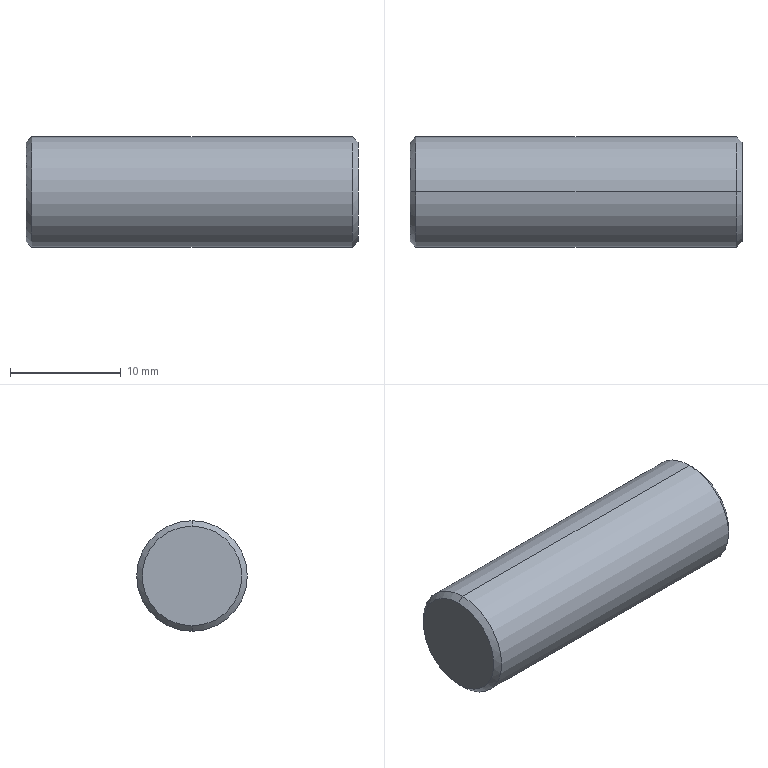Part | STEP file | LOCK PIN(LOCK PIN(Φ10×30)) | 1 solid | 12 faces | box 30 x 10 x 10 mm | volume 2277 mm3 | cone 6 | cylinder 4 | plane 2 | commonest cylinder face diameters 3.3 x2 10 x2